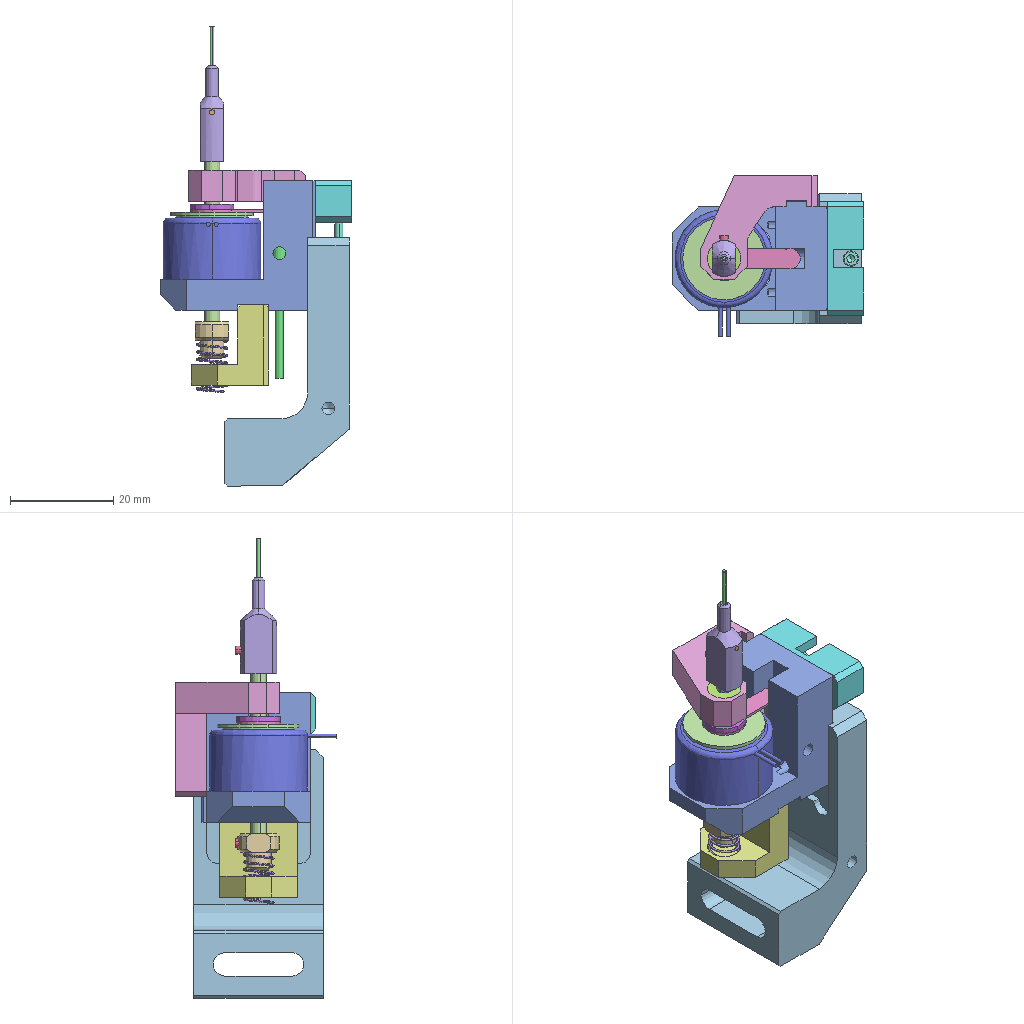Assembly | SolidWorks | 18 different items | 21 placed | box 37 x 31 x 89 mm
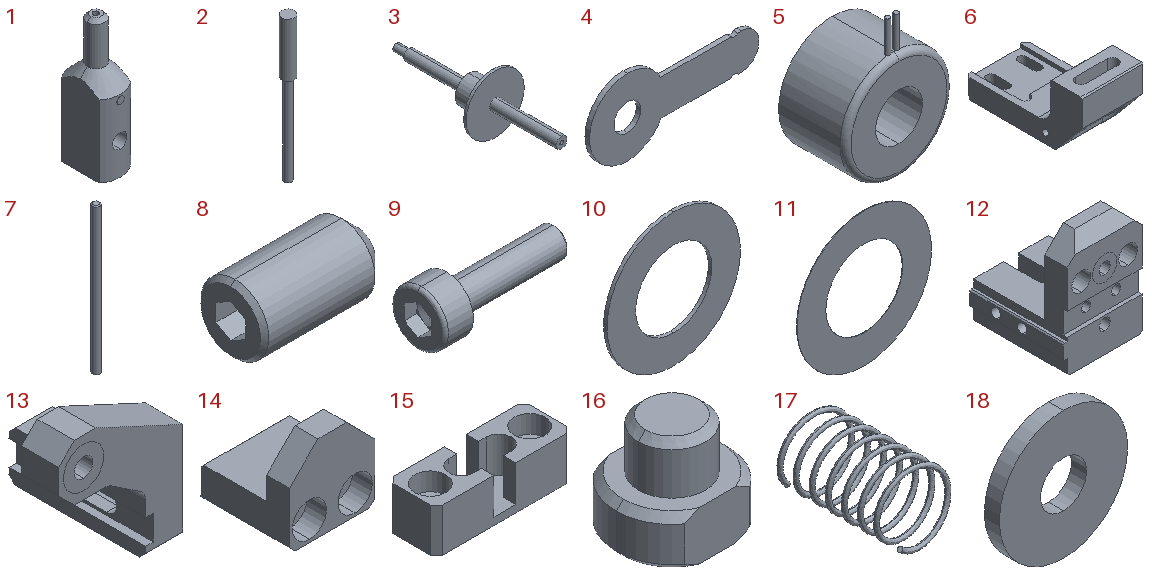Parts list (item | quantity | size | volume | features):
1 | x1 | 4.5 x 7 x 18.5 mm | 294.57 mm3 | features ICE 7, Chamfer 2, Extrusion 1, HoleWzd 1
2 | x1 | 2.8 x 2.8 x 32 mm | 114.103 mm3 | features Extrusion 1, ICE 1
3 | x1 | 16 x 45.5 x 16 mm | 652.862 mm3 | features ICE 2, Revolution 1
4 | x1 | 19 x 0.5 x 8.5 mm | 45.209 mm3 | features Extrusion 1, ICE 1
5 | x1 | 18.9 x 11.8 x 24.45 mm | 2887 mm3 | features ICE 2, HoleWzd 1, Revolution 1
6 | x1 | 25 x 48 x 24 mm | 9769 mm3 | features ICE 4, Cut 3, Chamfer 2, HoleWzd 2, Extrusion 1, Fillet 1, MirrorPattern 1
7 | x1 | 0.8 x 0.8 x 16.2 mm | 8.12 mm3 | features Chamfer 1, Extrusion 1
8 | x2 | 3 x 1.6 x 1.6 mm | 5.35 mm3 | features RevCut 2, Cut 1, LPattern 1, Revolution 1
9 | x3 | 7.6 x 3 x 3 mm | 21.652 mm3 | features Fillet 2, RevCut 2, Boss 1, Chamfer 1, Cut 1, Extrusion 1, LPattern 1
10 | x1 | 14 x 0.35 x 14 mm | 36.285 mm3 | features Extrusion 1
11 | x1 | 14 x 0.05 x 14 mm | 5.184 mm3 | features Extrusion 1
12 | x1 | 21 x 25 x 30 mm | 6312 mm3 | features ICE 7, HoleWzd 6, Chamfer 4, Cut 1, Extrusion 1
13 | x1 | 20 x 22 x 22.5 mm | 1597 mm3 | features ICE 10, Chamfer 2, Cut 1, Extrusion 1, Fillet 1
14 | x1 | 15 x 15.5 x 15 mm | 1371 mm3 | features Chamfer 3, ICE 3, Extrusion 1, HoleWzd 1
15 | x1 | 22 x 8 x 7 mm | 756.67 mm3 | features Chamfer 1, Extrusion 1, HoleWzd 1, ICE 1
16 | x1 | 8 x 6.5 x 7 mm | 166.104 mm3 | features ICE 3, Chamfer 1, Extrusion 1, HoleWzd 1
17 | x1 | 6 x 10.399 x 6 mm | 15.53 mm3 | features Helix 1, RefAxis 1, Sweep 1
18 | x1 | 8.5 x 1 x 8.5 mm | 49.439 mm3 | features Extrusion 1
Mates (type | each side: item.copy, entity, surface, feature):
Concentric | 5.1 face cylinder Revolve1 | 3.1 face cylinder Revolve1
Concentric | 3.1 face cylinder Revolve1 | 4.1 face cylinder Boss-Extrude1
Coincident | 3.1 face plane Revolve1 | 4.1 face plane Boss-Extrude1
Concentric | 6.1 face cylinder M3 Tapped Hole1 | 9.1 face cylinder BaseBody
Coincident | 15.1 face plane Cut-Extrude1 | 9.1 face plane BaseHead
Concentric | 3.1 face cylinder Revolve1 | 16.1 face cylinder Boss-Extrude1
Coincident | 11.1 face plane Boss-Extrude1 | 10.1 face plane Boss-Extrude1
Concentric | 11.1 face cylinder Boss-Extrude1 | 10.1 face cylinder Boss-Extrude1
Concentric | 10.1 face cylinder Boss-Extrude1 | 18.1 face cylinder Boss-Extrude1
Coincident | 5.1 face plane Revolve1 | 11.1 face plane Boss-Extrude1
Concentric | 5.1 face cylinder Revolve1 | 10.1 face cylinder Boss-Extrude1
Coincident | 4.1 face plane Boss-Extrude1 | 18.1 face plane Boss-Extrude1
Coincident | 3.1 face plane Revolve1 | 16.1 face plane Cut-Extrude1
Concentric | 3.1 face cylinder Revolve1 | 17.1 axis
Coincident | 16.1 face plane Boss-Extrude1 | 17.1 plane
LimitDistanceDim | 3.1 face plane Revolve1 | 10.1 face plane Boss-Extrude1
Concentric | 16.1 face cylinder M2.5 Tapped Hole1 | 8.1 face cylinder Base
Tangent | 3.1 face cylinder Revolve1 | 8.1 face plane Base
Concentric | 1.1 face cylinder Boss-Extrude2 | 7.1 face cylinder Boss-Extrude1
Tangent | 1.1 face cylinder Boss-Extrude3 | 7.1 face plane Boss-Extrude1
Concentric | 1.1 face cylinder M2.5 Tapped Hole1 | 8.2 face cylinder Base
Coincident | 3.1 face plane Revolve1 | 1.1 face plane Cut-Extrude2
Concentric | 3.1 face cylinder Revolve1 | 1.1 face cylinder Boss-Extrude1
Coincident | 12.1 face plane Boss-Extrude1 | 13.1 face plane Cut-Extrude3
DistanceDim | 13.1 face plane Boss-Extrude1 | 12.1 face plane Boss-Extrude1 | 2 times
Concentric | 12.1 face cylinder M3 Tapped Hole1 | 9.2 face cylinder BaseBody
Concentric | 12.1 face cylinder M3 Tapped Hole1 | 9.3 face cylinder BaseBody
Coincident | 13.1 face plane Cut-Extrude7 | 9.2 face plane BaseHead
Coincident | 9.2 face plane BaseHead | 9.3 face plane BaseHead
DistanceDim | 12.1 face plane Boss-Extrude1 | 6.1 face plane Boss-Extrude1
Coincident | 6.1 face plane Cut-Extrude1 | 12.1 face plane Boss-Extrude1 | 2 times
Concentric | 15.1 face cylinder Hole size per socket head cap screw type 1 | 12.1 face cylinder M2.5 Tapped Hole1
Concentric | 5.1 face cylinder Revolve1 | 12.1 face cylinder Boss-Extrude3
Parallel | 4.1 face plane Boss-Extrude1 | 12.1 face plane Cut-Extrude1
Coincident | 15.1 face plane Boss-Extrude1 | 12.1 face plane Boss-Extrude1
Coincident | 5.1 face plane Revolve1 | 12.1 face plane Boss-Extrude2
Coincident | 14.1 face plane Boss-Extrude1 | 12.1 face plane Cut-Extrude5
Width | 14.1 face plane Boss-Extrude1 | 14.1 face plane Boss-Extrude1 | 12.1 face plane Boss-Extrude1 | 12.1 face plane Boss-Extrude1
DistanceDim | 14.1 face plane Boss-Extrude1 | 12.1 face plane Boss-Extrude2
Parallel | 12.1 face plane Boss-Extrude2 | 16.1 face plane Cut-Extrude2
DistanceDim | 2.1 face plane Boss-Extrude1 | 12.1 face plane Boss-Extrude1
Concentric | 12.1 face cylinder Cut-Extrude9 | 2.1 face cylinder Boss-Extrude1
Parallel | 13.1 face plane Boss-Extrude2 | 1.1 face plane Cut-Extrude4